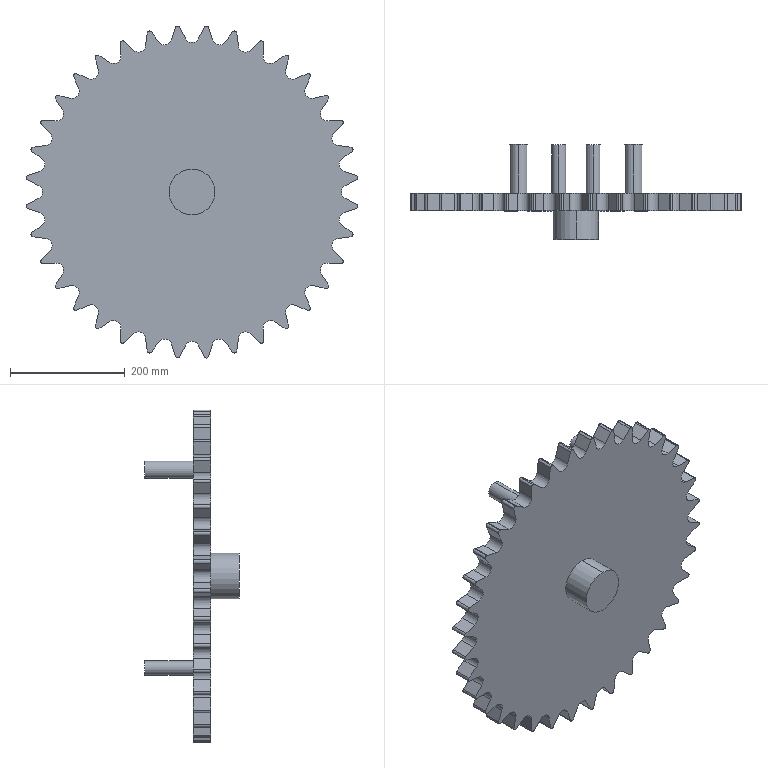Part | SolidWorks | features ICE 3, Extrusion 1 | 1 solid | 188 faces | box 577.823 x 165 x 577.823 mm | volume 7420375 mm3 | cylinder 109 | plane 79 | commonest cylinder face diameters 25 x53 8 x50 30 x4 80 x2